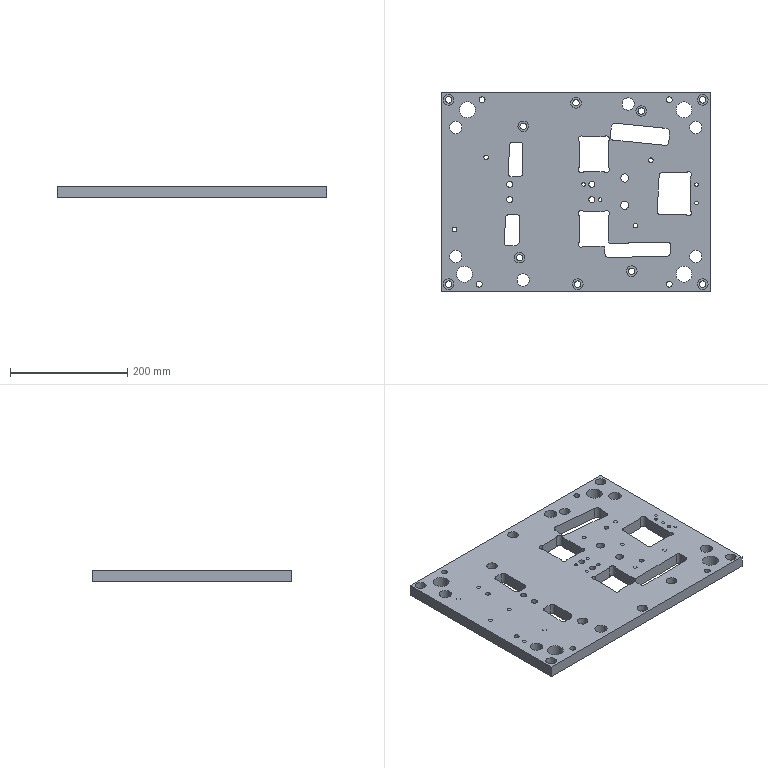Part | NX | features LIN_SOLID_COLOR 2 | 1 solid | 152 faces | box 460 x 340 x 20 mm | volume 2606427 mm3 | cylinder 92 | plane 60 | commonest cylinder face diameters 10 x26 6.8 x11 11 x10 18 x10 14 x7 21 x6